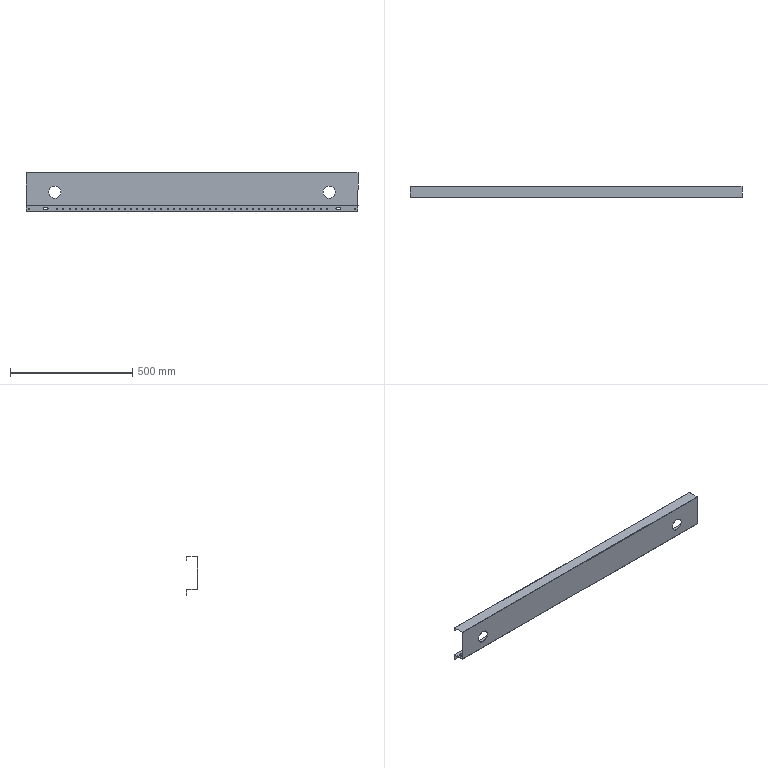Part | SolidWorks | features Cut 5, EdgeFlange 4, SMBaseFlange 2, FlatPattern 1, MirrorPattern 1, SheetMetal 1 | 1 solid | 162 faces | box 1356 x 46 x 159 mm | volume 347836 mm3 | cylinder 128 | plane 34 | commonest cylinder face diameters 4.2 x98 20 x14 0.4 x4 2.4 x4 10 x4 50 x4